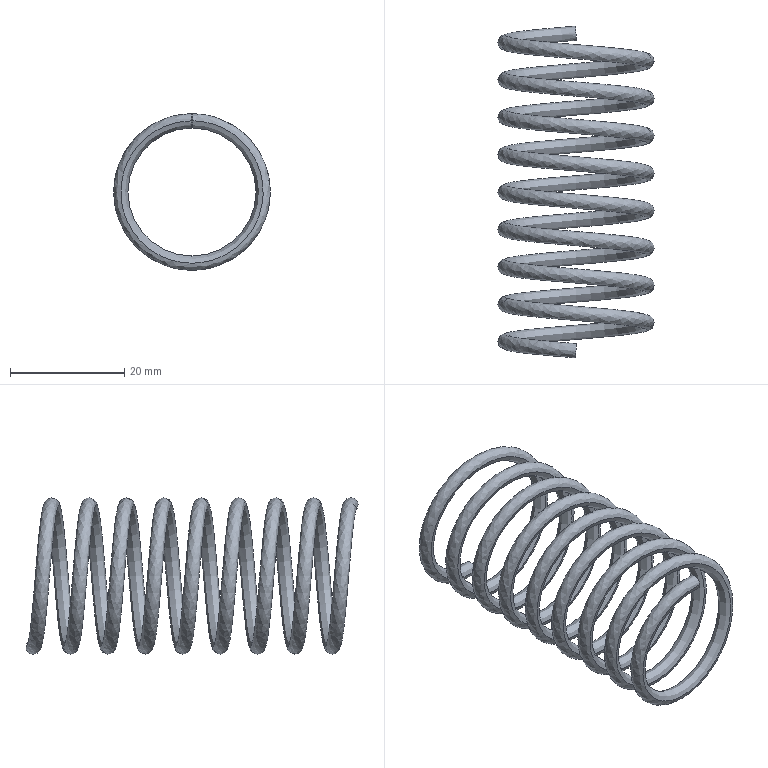Part | SolidWorks | features Helix 1, Sweep 1 | 1 solid | 4 faces | box 27.466 x 58.241 x 27.466 mm | volume 3289 mm3 | spline 2 | plane 2